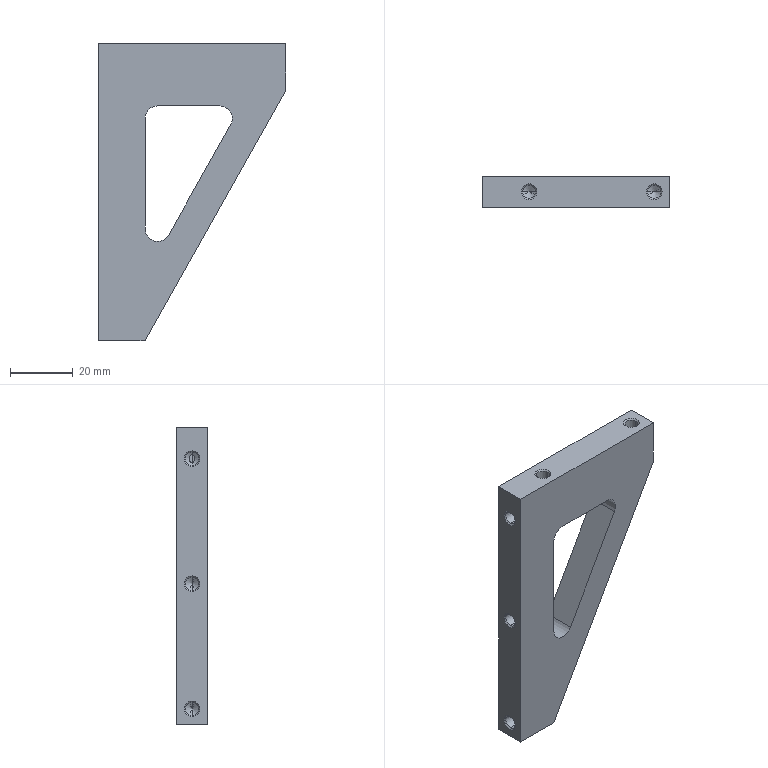Part | STEP file | B1-016 | 1 solid | 43 faces | box 60 x 10 x 95 mm | volume 30263 mm3 | cone 20 | cylinder 13 | plane 10 | commonest cylinder face diameters 4.2 x10 8 x3